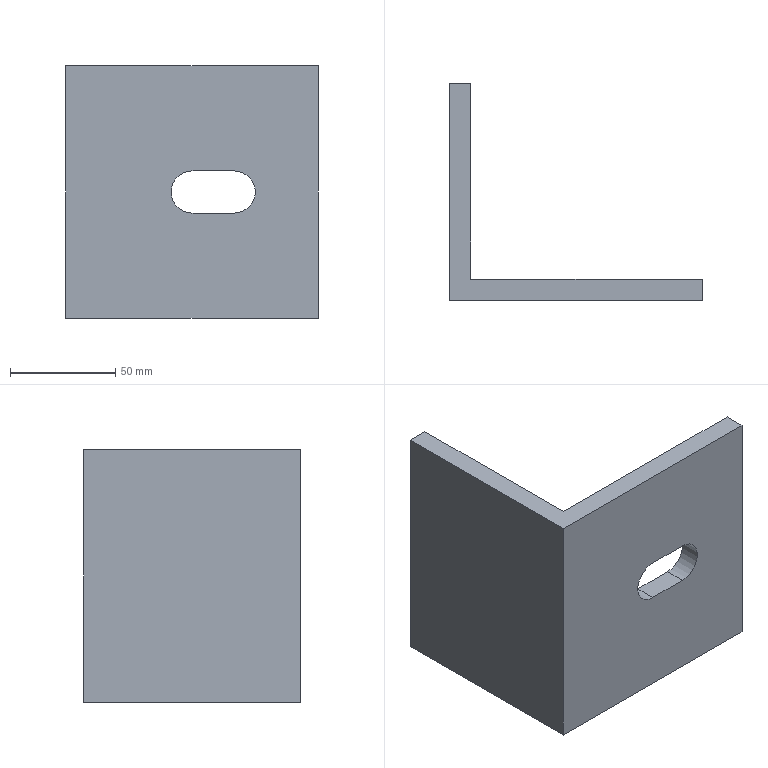Part | SolidWorks | features ExtruThin 1, ICE 1 | 1 solid | 12 faces | box 120 x 103 x 120 mm | volume 248458 mm3 | plane 10 | cylinder 2 | commonest cylinder face diameters 20 x2
STEP:
#1=CARTESIAN_POINT('',(80.,0.,-10.));
#2=VERTEX_POINT('',#1);
#3=CARTESIAN_POINT('',(60.,0.,-10.));
#4=VERTEX_POINT('',#3);
#5=CARTESIAN_POINT('',(60.,0.,-10.));
#6=DIRECTION('',(-1.,0.,0.));
#7=VECTOR('',#6,1000.);
#8=LINE('',#5,#7);
#9=EDGE_CURVE('',#2,#4,#8,.T.);
#10=ORIENTED_EDGE('',*,*,#9,.T.);
#11=CARTESIAN_POINT('',(60.,0.,10.));
#12=VERTEX_POINT('',#11);
#13=CARTESIAN_POINT('',(60.,0.,0.));
#14=DIRECTION('',(0.,1.,0.));
#15=DIRECTION('',(0.,0.,1.));
#16=AXIS2_PLACEMENT_3D('',#13,#14,#15);
#17=CIRCLE('',#16,10.);
#18=EDGE_CURVE('',#4,#12,#17,.T.);
#19=ORIENTED_EDGE('',*,*,#18,.T.);
#20=CARTESIAN_POINT('',(80.,0.,10.));
#21=VERTEX_POINT('',#20);
#22=CARTESIAN_POINT('',(60.,0.,10.));
#23=DIRECTION('',(1.,0.,0.));
#24=VECTOR('',#23,1000.);
#25=LINE('',#22,#24);
#26=EDGE_CURVE('',#12,#21,#25,.T.);
#27=ORIENTED_EDGE('',*,*,#26,.T.);
#28=CARTESIAN_POINT('',(80.,0.,0.));
#29=DIRECTION('',(0.,1.,0.));
#30=DIRECTION('',(0.,0.,1.));
#31=AXIS2_PLACEMENT_3D('',#28,#29,#30);
#32=CIRCLE('',#31,10.);
#33=EDGE_CURVE('',#21,#2,#32,.T.);
#34=ORIENTED_EDGE('',*,*,#33,.T.);
#35=EDGE_LOOP('',(#10,#19,#27,#34));
#36=FACE_BOUND('',#35,.T.);
#37=CARTESIAN_POINT('',(0.,0.,-60.));
#38=VERTEX_POINT('',#37);
#39=CARTESIAN_POINT('',(120.,0.,-60.));
#40=VERTEX_POINT('',#39);
#41=CARTESIAN_POINT('',(0.,0.,-60.));
#42=DIRECTION('',(1.,0.,0.));
#43=VECTOR('',#42,1000.);
#44=LINE('',#41,#43);
#45=EDGE_CURVE('',#38,#40,#44,.T.);
#46=ORIENTED_EDGE('',*,*,#45,.T.);
#47=CARTESIAN_POINT('',(120.,0.,60.));
#48=VERTEX_POINT('',#47);
#49=CARTESIAN_POINT('',(120.,0.,60.));
#50=DIRECTION('',(0.,0.,-1.));
#51=VECTOR('',#50,1000.);
#52=LINE('',#49,#51);
#53=EDGE_CURVE('',#48,#40,#52,.T.);
#54=ORIENTED_EDGE('',*,*,#53,.F.);
#55=CARTESIAN_POINT('',(0.,0.,60.));
#56=VERTEX_POINT('',#55);
#57=CARTESIAN_POINT('',(0.,0.,60.));
#58=DIRECTION('',(1.,0.,0.));
#59=VECTOR('',#58,1000.);
#60=LINE('',#57,#59);
#61=EDGE_CURVE('',#56,#48,#60,.T.);
#62=ORIENTED_EDGE('',*,*,#61,.F.);
#63=CARTESIAN_POINT('',(0.,0.,60.));
#64=DIRECTION('',(0.,0.,-1.));
#65=VECTOR('',#64,1000.);
#66=LINE('',#63,#65);
#67=EDGE_CURVE('',#56,#38,#66,.T.);
#68=ORIENTED_EDGE('',*,*,#67,.T.);
#69=EDGE_LOOP('',(#46,#54,#62,#68));
#70=FACE_OUTER_BOUND('',#69,.T.);
#71=CARTESIAN_POINT('',(0.,0.,60.));
#72=DIRECTION('',(0.,1.,0.));
#73=DIRECTION('',(0.,0.,1.));
#74=AXIS2_PLACEMENT_3D('',#71,#72,#73);
#75=PLANE('',#74);
#76=ADVANCED_FACE('',(#36,#70),#75,.F.);
#77=CARTESIAN_POINT('',(120.,10.,-60.));
#78=VERTEX_POINT('',#77);
#79=CARTESIAN_POINT('',(120.,10.,-60.));
#80=DIRECTION('',(0.,-1.,0.));
#81=VECTOR('',#80,1000.);
#82=LINE('',#79,#81);
#83=EDGE_CURVE('',#78,#40,#82,.T.);
#84=ORIENTED_EDGE('',*,*,#83,.F.);
#85=CARTESIAN_POINT('',(120.,10.,60.));
#86=VERTEX_POINT('',#85);
#87=CARTESIAN_POINT('',(120.,10.,60.));
#88=DIRECTION('',(0.,0.,-1.));
#89=VECTOR('',#88,1000.);
#90=LINE('',#87,#89);
#91=EDGE_CURVE('',#86,#78,#90,.T.);
#92=ORIENTED_EDGE('',*,*,#91,.F.);
#93=CARTESIAN_POINT('',(120.,10.,60.));
#94=DIRECTION('',(0.,-1.,0.));
#95=VECTOR('',#94,1000.);
#96=LINE('',#93,#95);
#97=EDGE_CURVE('',#86,#48,#96,.T.);
#98=ORIENTED_EDGE('',*,*,#97,.T.);
#99=ORIENTED_EDGE('',*,*,#53,.T.);
#100=EDGE_LOOP('',(#84,#92,#98,#99));
#101=FACE_OUTER_BOUND('',#100,.T.);
#102=CARTESIAN_POINT('',(120.,10.,60.));
#103=DIRECTION('',(1.,0.,0.));
#104=DIRECTION('',(0.,0.,-1.));
#105=AXIS2_PLACEMENT_3D('',#102,#103,#104);
#106=PLANE('',#105);
#107=ADVANCED_FACE('',(#101),#106,.T.);
#108=CARTESIAN_POINT('',(60.,10.,-10.));
#109=VERTEX_POINT('',#108);
#110=CARTESIAN_POINT('',(60.,10.,10.));
#111=VERTEX_POINT('',#110);
#112=CARTESIAN_POINT('',(60.,10.,0.));
#113=DIRECTION('',(0.,1.,0.));
#114=DIRECTION('',(0.,0.,1.));
#115=AXIS2_PLACEMENT_3D('',#112,#113,#114);
#116=CIRCLE('',#115,10.);
#117=EDGE_CURVE('',#109,#111,#116,.T.);
#118=ORIENTED_EDGE('',*,*,#117,.F.);
#119=CARTESIAN_POINT('',(80.,10.,-10.));
#120=VERTEX_POINT('',#119);
#121=CARTESIAN_POINT('',(60.,10.,-10.));
#122=DIRECTION('',(-1.,0.,0.));
#123=VECTOR('',#122,1000.);
#124=LINE('',#121,#123);
#125=EDGE_CURVE('',#120,#109,#124,.T.);
#126=ORIENTED_EDGE('',*,*,#125,.F.);
#127=CARTESIAN_POINT('',(80.,10.,10.));
#128=VERTEX_POINT('',#127);
#129=CARTESIAN_POINT('',(80.,10.,0.));
#130=DIRECTION('',(0.,1.,0.));
#131=DIRECTION('',(0.,0.,1.));
#132=AXIS2_PLACEMENT_3D('',#129,#130,#131);
#133=CIRCLE('',#132,10.);
#134=EDGE_CURVE('',#128,#120,#133,.T.);
#135=ORIENTED_EDGE('',*,*,#134,.F.);
#136=CARTESIAN_POINT('',(60.,10.,10.));
#137=DIRECTION('',(1.,0.,0.));
#138=VECTOR('',#137,1000.);
#139=LINE('',#136,#138);
#140=EDGE_CURVE('',#111,#128,#139,.T.);
#141=ORIENTED_EDGE('',*,*,#140,.F.);
#142=EDGE_LOOP('',(#118,#126,#135,#141));
#143=FACE_BOUND('',#142,.T.);
#144=CARTESIAN_POINT('',(10.,10.,-60.));
#145=VERTEX_POINT('',#144);
#146=CARTESIAN_POINT('',(0.,10.,-60.));
#147=DIRECTION('',(1.,0.,0.));
#148=VECTOR('',#147,1000.);
#149=LINE('',#146,#148);
#150=EDGE_CURVE('',#145,#78,#149,.T.);
#151=ORIENTED_EDGE('',*,*,#150,.F.);
#152=CARTESIAN_POINT('',(10.,10.,60.));
#153=VERTEX_POINT('',#152);
#154=CARTESIAN_POINT('',(10.,10.,60.));
#155=DIRECTION('',(0.,0.,-1.));
#156=VECTOR('',#155,1000.);
#157=LINE('',#154,#156);
#158=EDGE_CURVE('',#153,#145,#157,.T.);
#159=ORIENTED_EDGE('',*,*,#158,.F.);
#160=CARTESIAN_POINT('',(0.,10.,60.));
#161=DIRECTION('',(1.,0.,0.));
#162=VECTOR('',#161,1000.);
#163=LINE('',#160,#162);
#164=EDGE_CURVE('',#153,#86,#163,.T.);
#165=ORIENTED_EDGE('',*,*,#164,.T.);
#166=ORIENTED_EDGE('',*,*,#91,.T.);
#167=EDGE_LOOP('',(#151,#159,#165,#166));
#168=FACE_OUTER_BOUND('',#167,.T.);
#169=CARTESIAN_POINT('',(0.,10.,60.));
#170=DIRECTION('',(0.,1.,0.));
#171=DIRECTION('',(0.,0.,1.));
#172=AXIS2_PLACEMENT_3D('',#169,#170,#171);
#173=PLANE('',#172);
#174=ADVANCED_FACE('',(#143,#168),#173,.T.);
#175=CARTESIAN_POINT('',(10.,103.,-60.));
#176=VERTEX_POINT('',#175);
#177=CARTESIAN_POINT('',(10.,0.,-60.));
#178=DIRECTION('',(0.,-1.,0.));
#179=VECTOR('',#178,1000.);
#180=LINE('',#177,#179);
#181=EDGE_CURVE('',#176,#145,#180,.T.);
#182=ORIENTED_EDGE('',*,*,#181,.F.);
#183=CARTESIAN_POINT('',(10.,103.,60.));
#184=VERTEX_POINT('',#183);
#185=CARTESIAN_POINT('',(10.,103.,60.));
#186=DIRECTION('',(0.,0.,-1.));
#187=VECTOR('',#186,1000.);
#188=LINE('',#185,#187);
#189=EDGE_CURVE('',#184,#176,#188,.T.);
#190=ORIENTED_EDGE('',*,*,#189,.F.);
#191=CARTESIAN_POINT('',(10.,0.,60.));
#192=DIRECTION('',(0.,-1.,0.));
#193=VECTOR('',#192,1000.);
#194=LINE('',#191,#193);
#195=EDGE_CURVE('',#184,#153,#194,.T.);
#196=ORIENTED_EDGE('',*,*,#195,.T.);
#197=ORIENTED_EDGE('',*,*,#158,.T.);
#198=EDGE_LOOP('',(#182,#190,#196,#197));
#199=FACE_OUTER_BOUND('',#198,.T.);
#200=CARTESIAN_POINT('',(10.,0.,60.));
#201=DIRECTION('',(1.,0.,0.));
#202=DIRECTION('',(0.,0.,-1.));
#203=AXIS2_PLACEMENT_3D('',#200,#201,#202);
#204=PLANE('',#203);
#205=ADVANCED_FACE('',(#199),#204,.T.);
#206=CARTESIAN_POINT('',(0.,103.,-60.));
#207=VERTEX_POINT('',#206);
#208=CARTESIAN_POINT('',(0.,103.,-60.));
#209=DIRECTION('',(1.,0.,0.));
#210=VECTOR('',#209,1000.);
#211=LINE('',#208,#210);
#212=EDGE_CURVE('',#207,#176,#211,.T.);
#213=ORIENTED_EDGE('',*,*,#212,.F.);
#214=CARTESIAN_POINT('',(0.,103.,60.));
#215=VERTEX_POINT('',#214);
#216=CARTESIAN_POINT('',(0.,103.,60.));
#217=DIRECTION('',(0.,0.,-1.));
#218=VECTOR('',#217,1000.);
#219=LINE('',#216,#218);
#220=EDGE_CURVE('',#215,#207,#219,.T.);
#221=ORIENTED_EDGE('',*,*,#220,.F.);
#222=CARTESIAN_POINT('',(0.,103.,60.));
#223=DIRECTION('',(1.,0.,0.));
#224=VECTOR('',#223,1000.);
#225=LINE('',#222,#224);
#226=EDGE_CURVE('',#215,#184,#225,.T.);
#227=ORIENTED_EDGE('',*,*,#226,.T.);
#228=ORIENTED_EDGE('',*,*,#189,.T.);
#229=EDGE_LOOP('',(#213,#221,#227,#228));
#230=FACE_OUTER_BOUND('',#229,.T.);
#231=CARTESIAN_POINT('',(0.,103.,60.));
#232=DIRECTION('',(0.,1.,0.));
#233=DIRECTION('',(0.,0.,1.));
#234=AXIS2_PLACEMENT_3D('',#231,#232,#233);
#235=PLANE('',#234);
#236=ADVANCED_FACE('',(#230),#235,.T.);
#237=CARTESIAN_POINT('',(0.,0.,-60.));
#238=DIRECTION('',(0.,-1.,0.));
#239=VECTOR('',#238,1000.);
#240=LINE('',#237,#239);
#241=EDGE_CURVE('',#207,#38,#240,.T.);
#242=ORIENTED_EDGE('',*,*,#241,.T.);
#243=ORIENTED_EDGE('',*,*,#67,.F.);
#244=CARTESIAN_POINT('',(0.,0.,60.));
#245=DIRECTION('',(0.,-1.,0.));
#246=VECTOR('',#245,1000.);
#247=LINE('',#244,#246);
#248=EDGE_CURVE('',#215,#56,#247,.T.);
#249=ORIENTED_EDGE('',*,*,#248,.F.);
#250=ORIENTED_EDGE('',*,*,#220,.T.);
#251=EDGE_LOOP('',(#242,#243,#249,#250));
#252=FACE_OUTER_BOUND('',#251,.T.);
#253=CARTESIAN_POINT('',(0.,0.,60.));
#254=DIRECTION('',(1.,0.,0.));
#255=DIRECTION('',(0.,0.,-1.));
#256=AXIS2_PLACEMENT_3D('',#253,#254,#255);
#257=PLANE('',#256);
#258=ADVANCED_FACE('',(#252),#257,.F.);
#259=ORIENTED_EDGE('',*,*,#61,.T.);
#260=ORIENTED_EDGE('',*,*,#97,.F.);
#261=ORIENTED_EDGE('',*,*,#164,.F.);
#262=ORIENTED_EDGE('',*,*,#195,.F.);
#263=ORIENTED_EDGE('',*,*,#226,.F.);
#264=ORIENTED_EDGE('',*,*,#248,.T.);
#265=EDGE_LOOP('',(#259,#260,#261,#262,#263,#264));
#266=FACE_OUTER_BOUND('',#265,.T.);
#267=CARTESIAN_POINT('',(0.,0.,60.));
#268=DIRECTION('',(0.,0.,-1.));
#269=DIRECTION('',(-1.,0.,0.));
#270=AXIS2_PLACEMENT_3D('',#267,#268,#269);
#271=PLANE('',#270);
#272=ADVANCED_FACE('',(#266),#271,.F.);
#273=ORIENTED_EDGE('',*,*,#45,.F.);
#274=ORIENTED_EDGE('',*,*,#241,.F.);
#275=ORIENTED_EDGE('',*,*,#212,.T.);
#276=ORIENTED_EDGE('',*,*,#181,.T.);
#277=ORIENTED_EDGE('',*,*,#150,.T.);
#278=ORIENTED_EDGE('',*,*,#83,.T.);
#279=EDGE_LOOP('',(#273,#274,#275,#276,#277,#278));
#280=FACE_OUTER_BOUND('',#279,.T.);
#281=CARTESIAN_POINT('',(0.,0.,-60.));
#282=DIRECTION('',(0.,0.,-1.));
#283=DIRECTION('',(-1.,0.,0.));
#284=AXIS2_PLACEMENT_3D('',#281,#282,#283);
#285=PLANE('',#284);
#286=ADVANCED_FACE('',(#280),#285,.T.);
#287=ORIENTED_EDGE('',*,*,#117,.T.);
#288=CARTESIAN_POINT('',(60.,0.,10.));
#289=DIRECTION('',(0.,1.,0.));
#290=VECTOR('',#289,1000.);
#291=LINE('',#288,#290);
#292=EDGE_CURVE('',#12,#111,#291,.T.);
#293=ORIENTED_EDGE('',*,*,#292,.F.);
#294=ORIENTED_EDGE('',*,*,#18,.F.);
#295=CARTESIAN_POINT('',(60.,0.,-10.));
#296=DIRECTION('',(0.,1.,0.));
#297=VECTOR('',#296,1000.);
#298=LINE('',#295,#297);
#299=EDGE_CURVE('',#4,#109,#298,.T.);
#300=ORIENTED_EDGE('',*,*,#299,.T.);
#301=EDGE_LOOP('',(#287,#293,#294,#300));
#302=FACE_OUTER_BOUND('',#301,.T.);
#303=CARTESIAN_POINT('',(60.,0.,0.));
#304=DIRECTION('',(0.,1.,0.));
#305=DIRECTION('',(0.,0.,1.));
#306=AXIS2_PLACEMENT_3D('',#303,#304,#305);
#307=CYLINDRICAL_SURFACE('',#306,10.);
#308=ADVANCED_FACE('',(#302),#307,.F.);
#309=ORIENTED_EDGE('',*,*,#125,.T.);
#310=ORIENTED_EDGE('',*,*,#299,.F.);
#311=ORIENTED_EDGE('',*,*,#9,.F.);
#312=CARTESIAN_POINT('',(80.,0.,-10.));
#313=DIRECTION('',(0.,1.,0.));
#314=VECTOR('',#313,1000.);
#315=LINE('',#312,#314);
#316=EDGE_CURVE('',#2,#120,#315,.T.);
#317=ORIENTED_EDGE('',*,*,#316,.T.);
#318=EDGE_LOOP('',(#309,#310,#311,#317));
#319=FACE_OUTER_BOUND('',#318,.T.);
#320=CARTESIAN_POINT('',(60.,0.,-10.));
#321=DIRECTION('',(0.,0.,-1.));
#322=DIRECTION('',(-1.,0.,0.));
#323=AXIS2_PLACEMENT_3D('',#320,#321,#322);
#324=PLANE('',#323);
#325=ADVANCED_FACE('',(#319),#324,.F.);
#326=ORIENTED_EDGE('',*,*,#134,.T.);
#327=ORIENTED_EDGE('',*,*,#316,.F.);
#328=ORIENTED_EDGE('',*,*,#33,.F.);
#329=CARTESIAN_POINT('',(80.,0.,10.));
#330=DIRECTION('',(0.,1.,0.));
#331=VECTOR('',#330,1000.);
#332=LINE('',#329,#331);
#333=EDGE_CURVE('',#21,#128,#332,.T.);
#334=ORIENTED_EDGE('',*,*,#333,.T.);
#335=EDGE_LOOP('',(#326,#327,#328,#334));
#336=FACE_OUTER_BOUND('',#335,.T.);
#337=CARTESIAN_POINT('',(80.,0.,0.));
#338=DIRECTION('',(0.,1.,0.));
#339=DIRECTION('',(0.,0.,1.));
#340=AXIS2_PLACEMENT_3D('',#337,#338,#339);
#341=CYLINDRICAL_SURFACE('',#340,10.);
#342=ADVANCED_FACE('',(#336),#341,.F.);
#343=ORIENTED_EDGE('',*,*,#140,.T.);
#344=ORIENTED_EDGE('',*,*,#333,.F.);
#345=ORIENTED_EDGE('',*,*,#26,.F.);
#346=ORIENTED_EDGE('',*,*,#292,.T.);
#347=EDGE_LOOP('',(#343,#344,#345,#346));
#348=FACE_OUTER_BOUND('',#347,.T.);
#349=CARTESIAN_POINT('',(60.,0.,10.));
#350=DIRECTION('',(0.,0.,1.));
#351=DIRECTION('',(1.,0.,0.));
#352=AXIS2_PLACEMENT_3D('',#349,#350,#351);
#353=PLANE('',#352);
#354=ADVANCED_FACE('',(#348),#353,.F.);
#355=CLOSED_SHELL('',(#76,#107,#174,#205,#236,#258,#272,#286,#308,#325,#342,#354));
#356=MANIFOLD_SOLID_BREP('',#355);
#357=CARTESIAN_POINT('',(0.,0.,0.));
#358=DIRECTION('',(0.,0.,1.));
#359=DIRECTION('',(1.,0.,0.));
#360=AXIS2_PLACEMENT_3D('',#357,#358,#359);
#361=(LENGTH_UNIT()NAMED_UNIT(*)SI_UNIT(.MILLI.,.METRE.));
#362=UNCERTAINTY_MEASURE_WITH_UNIT(LENGTH_MEASURE(0.00001),#361,'','');
#363=(NAMED_UNIT(*)PLANE_ANGLE_UNIT()SI_UNIT($,.RADIAN.));
#364=(NAMED_UNIT(*)SI_UNIT($,.STERADIAN.)SOLID_ANGLE_UNIT());
#365=(GEOMETRIC_REPRESENTATION_CONTEXT(3)GLOBAL_UNCERTAINTY_ASSIGNED_CONTEXT((#362))GLOBAL_UNIT_ASSIGNED_CONTEXT((#361,#363,#364))REPRESENTATION_CONTEXT('',''));
#366=ADVANCED_BREP_SHAPE_REPRESENTATION('',(#356,#360),#365);